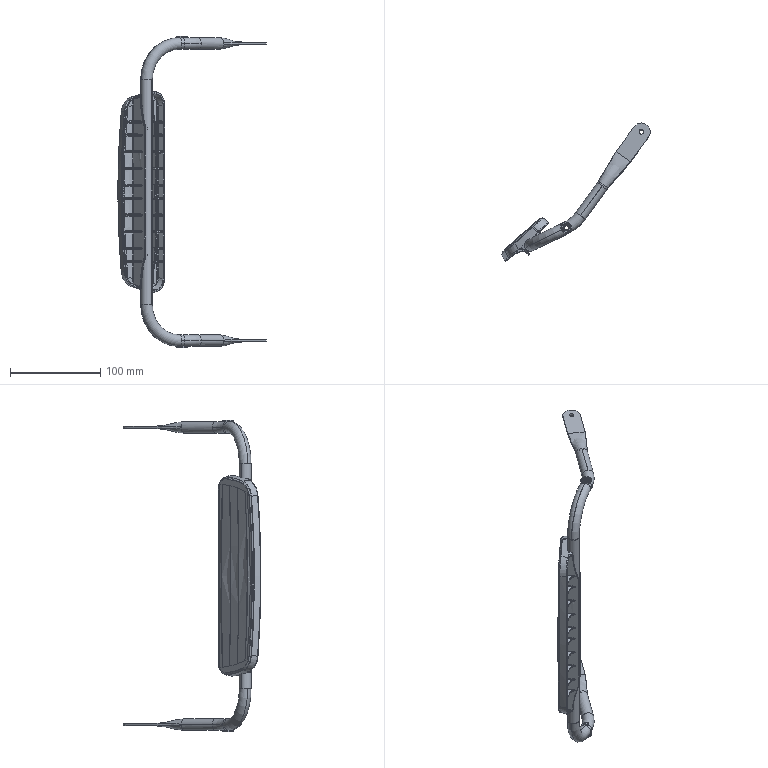Part | SolidWorks | 3 solids | 1167 faces | box 164.156 x 152.53 x 345 mm | volume 87735 mm3 | spline 489 | cylinder 424 | plane 194 | cone 44 | torus 16 | commonest cylinder face diameters 1 x315 1.2 x14 5.2 x12 13.5 x12 11.4 x10 13 x10